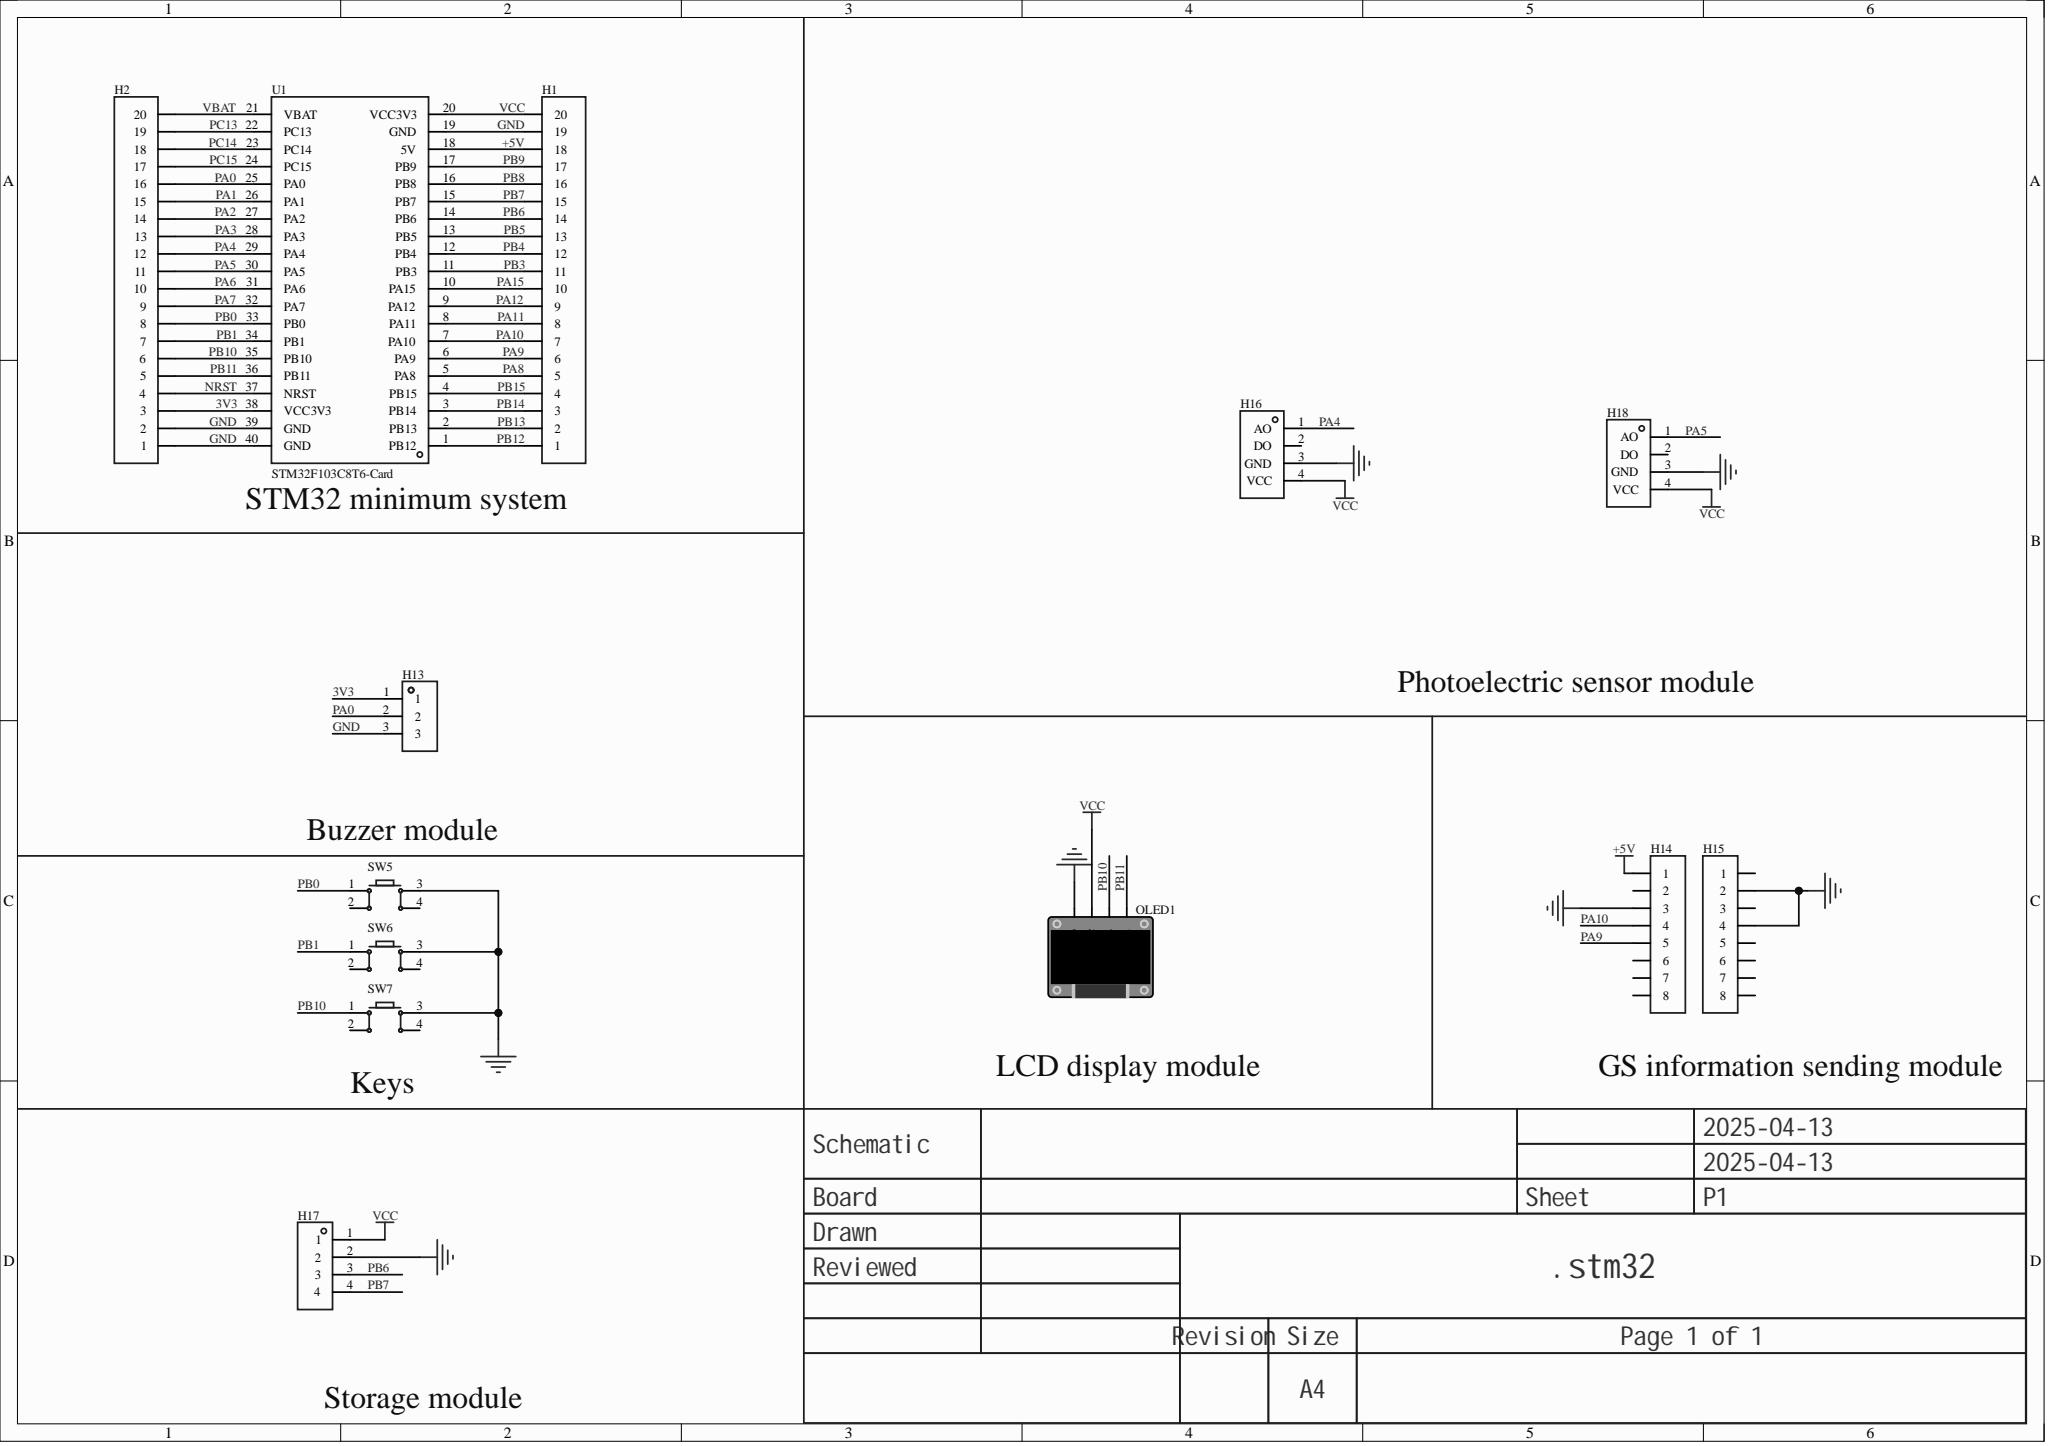Circuit board | Altium Designer | 13 parts | 38 nets
Bill of materials:
Comment,Description,Designator,Footprint,LibRef,Quantity
"","","H1, H2","HDR-TH_20P-P2.54-V-F","HDR-F_2.54_1x20P","2"
"","","H13","HDR-TH_3P-P2.54-V-F","HDR-F_2.54_1x3P","1"
"","","H14, H15","HDR-TH_8P-P2.54-V-F-1","HDR-F_2.54_1x8P","2"
"","","H16, H18","HDR-TH_4P-P2.54-V-F","HDR-F_2.54_1x4P","2"
"","","H17","HDR-TH_4P-P2.54-V-M","HDR-M_2.54_1x4P","1"
"","","OLED1","0.96OLED_4P","0.96OLED模块_4P","1"
"","","SW5, SW6, SW7","SW-TH_4P-L6.0-W6.0-P4.50-LS6.5","Key_TH_6x6x6","3"
"STM32F103C8T6-Card","","U1","CONN-TH_L53.3-W22.9_STM32F103C8T6-CARD","STM32F103C8T6-Card","1"
Netlist (Protel format):
[
H1
HDR-TH_20P-P2.54-V-F




]
[
H2
HDR-TH_20P-P2.54-V-F




]
[
H13
HDR-TH_3P-P2.54-V-F




]
[
H14
HDR-TH_8P-P2.54-V-F-1




]
[
H15
HDR-TH_8P-P2.54-V-F-1




]
[
H16
HDR-TH_4P-P2.54-V-F




]
[
H17
HDR-TH_4P-P2.54-V-M




]
[
H18
HDR-TH_4P-P2.54-V-F




]
[
OLED1
0.96OLED_4P




]
[
SW5
SW-TH_4P-L6.0-W6.0-P4.50-LS6.5




]
[
SW6
SW-TH_4P-L6.0-W6.0-P4.50-LS6.5




]
[
SW7
SW-TH_4P-L6.0-W6.0-P4.50-LS6.5




]
[
U1
CONN-TH_L53.3-W22.9_STM32F103C8T6-CARD
STM32F103C8T6-Card



]
(
VCC
H1-20
H16-4
H17-1
H18-4
OLED1-2
U1-20
)
(
VBAT
H2-20
U1-21
)
(
PC15
H2-17
U1-24
)
(
PC14
H2-18
U1-23
)
(
PC13
H2-19
U1-22
)
(
PB15
H1-4
U1-4
)
(
PB14
H1-3
U1-3
)
(
PB13
H1-2
U1-2
)
(
PB12
H1-1
U1-1
)
(
PB11
H2-5
OLED1-4
U1-36
)
(
PB10
H2-6
OLED1-3
SW7-1
U1-35
)
(
PB9
H1-17
U1-17
)
(
PB8
H1-16
U1-16
)
(
PB7
H1-15
H17-4
U1-15
)
(
PB6
H1-14
H17-3
U1-14
)
(
PB5
H1-13
U1-13
)
(
PB4
H1-12
U1-12
)
(
PB3
H1-11
U1-11
)
(
PB1
H2-7
SW6-1
U1-34
)
(
PB0
H2-8
SW5-1
U1-33
)
(
PA15
H1-10
U1-10
)
(
PA12
H1-9
U1-9
)
(
PA11
H1-8
U1-8
)
(
PA10
H1-7
H14-4
U1-7
)
(
PA9
H1-6
H14-5
U1-6
)
(
PA8
H1-5
U1-5
)
(
PA7
H2-9
U1-32
)
(
PA6
H2-10
U1-31
)
(
PA5
H2-11
H18-1
U1-30
)
(
PA4
H2-12
H16-1
U1-29
)
(
PA3
H2-13
U1-28
)
(
PA2
H2-14
U1-27
)
(
PA1
H2-15
U1-26
)
(
PA0
H2-16
H13-2
U1-25
)
(
NRST
H2-4
U1-37
)
(
GND
H1-19
H2-1
H2-2
H13-3
H14-3
H15-2
H15-4
H16-3
H17-2
H18-3
OLED1-1
SW5-3
SW6-3
SW7-3
U1-19
U1-39
U1-40
)
(
+5V
H1-18
H14-1
U1-18
)
(
3V3
H2-3
H13-1
U1-38
)